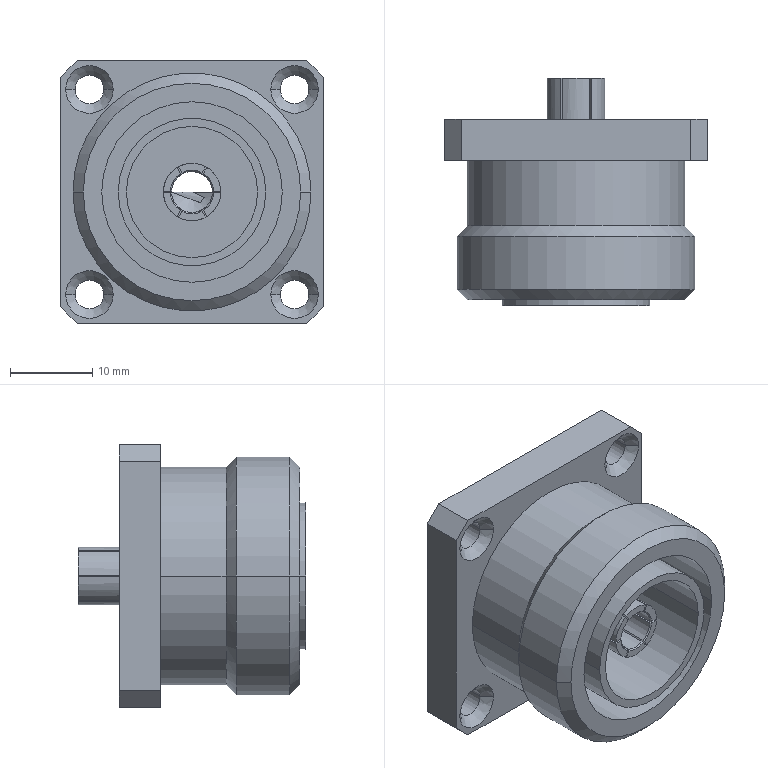Part | STEP file | Connector L29-50KFDA | 2 solids | 125 faces | box 32 x 27.7 x 32 mm | volume 10941 mm3 | plane 65 | cylinder 32 | cone 28 | commonest cylinder face diameters 3.5 x8 5 x8 7 x4 16 x4 18 x2 22 x2